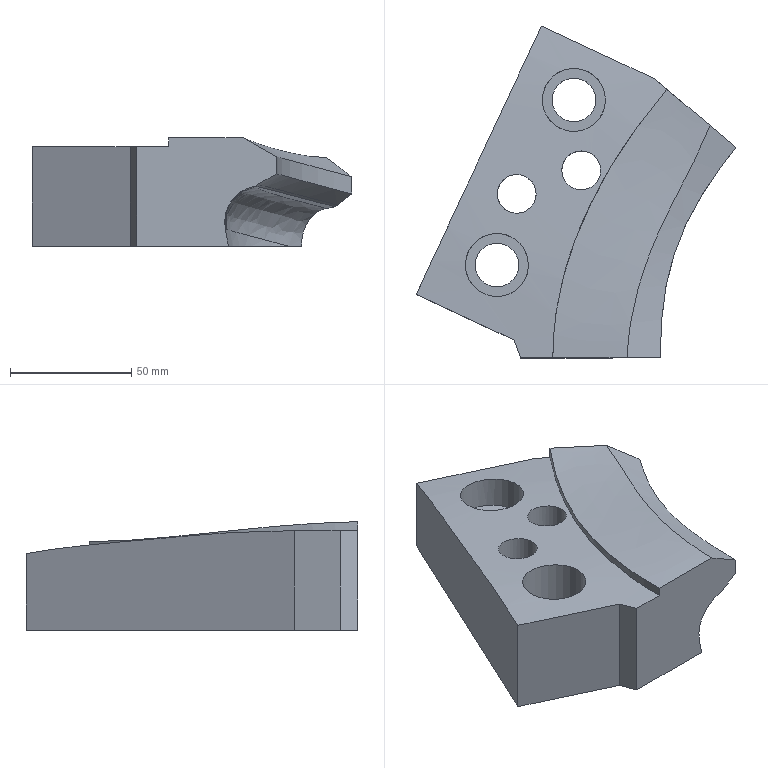Part | NX | features solid 2 | 1 solid | 25 faces | box 131.571 x 136.634 x 44.667 mm | volume 321257 mm3 | spline 10 | plane 9 | cylinder 6 | commonest cylinder face diameters 16 x2 18 x2 26 x2
STEP:
#1=CARTESIAN_POINT('',(-688.081,35.625,61.862));
#2=VERTEX_POINT('',#1);
#3=CARTESIAN_POINT('',(-693.271,39.979,61.591));
#4=VERTEX_POINT('',#3);
#5=CARTESIAN_POINT('',(-688.081,35.625,61.862));
#6=CARTESIAN_POINT('',(-689.811,37.076,61.773));
#7=CARTESIAN_POINT('',(-691.541,38.528,61.682));
#8=CARTESIAN_POINT('',(-693.271,39.979,61.591));
#9=B_SPLINE_CURVE_WITH_KNOTS('',3,(#5,#6,#7,#8),.UNSPECIFIED.,.F.,.F.,(4,4),(0.02865,0.03543),.UNSPECIFIED.);
#10=EDGE_CURVE('',#2,#4,#9,.T.);
#11=ORIENTED_EDGE('',*,*,#10,.F.);
#12=CARTESIAN_POINT('',(-688.081,35.625,66.502));
#13=VERTEX_POINT('',#12);
#14=CARTESIAN_POINT('',(-688.081,35.625,66.502));
#15=DIRECTION('',(0.,0.,1.));
#16=VECTOR('',#15,1000.);
#17=LINE('',#14,#16);
#18=EDGE_CURVE('',#2,#13,#17,.T.);
#19=ORIENTED_EDGE('',*,*,#18,.T.);
#20=CARTESIAN_POINT('',(-670.187,20.61,66.502));
#21=VERTEX_POINT('',#20);
#22=CARTESIAN_POINT('',(-688.081,35.625,66.502));
#23=CARTESIAN_POINT('',(-682.117,30.62,66.502));
#24=CARTESIAN_POINT('',(-676.152,25.615,66.502));
#25=CARTESIAN_POINT('',(-670.187,20.61,66.502));
#26=B_SPLINE_CURVE_WITH_KNOTS('',3,(#22,#23,#24,#25),.UNSPECIFIED.,.F.,.F.,(4,4),(0.006775,0.03013),.UNSPECIFIED.);
#27=EDGE_CURVE('',#13,#21,#26,.T.);
#28=ORIENTED_EDGE('',*,*,#27,.T.);
#29=CARTESIAN_POINT('',(-659.667,11.782,58.591));
#30=VERTEX_POINT('',#29);
#31=CARTESIAN_POINT('',(-670.187,20.61,66.502));
#32=CARTESIAN_POINT('',(-666.68,17.667,63.866));
#33=CARTESIAN_POINT('',(-663.173,14.724,61.229));
#34=CARTESIAN_POINT('',(-659.667,11.782,58.591));
#35=B_SPLINE_CURVE_WITH_KNOTS('',3,(#31,#32,#33,#34),.UNSPECIFIED.,.F.,.F.,(4,4),(0.001125,0.01697),.UNSPECIFIED.);
#36=EDGE_CURVE('',#21,#30,#35,.T.);
#37=ORIENTED_EDGE('',*,*,#36,.T.);
#38=CARTESIAN_POINT('',(-659.667,11.782,51.502));
#39=VERTEX_POINT('',#38);
#40=CARTESIAN_POINT('',(-659.667,11.782,58.342));
#41=DIRECTION('',(0.,0.,-1.));
#42=VECTOR('',#41,1000.);
#43=LINE('',#40,#42);
#44=EDGE_CURVE('',#30,#39,#43,.T.);
#45=ORIENTED_EDGE('',*,*,#44,.T.);
#46=CARTESIAN_POINT('',(-665.567,16.733,46.945));
#47=VERTEX_POINT('',#46);
#48=CARTESIAN_POINT('',(-665.567,16.733,46.945));
#49=CARTESIAN_POINT('',(-663.6,15.082,48.464));
#50=CARTESIAN_POINT('',(-661.633,13.432,49.982));
#51=CARTESIAN_POINT('',(-659.667,11.782,51.502));
#52=B_SPLINE_CURVE_WITH_KNOTS('',3,(#48,#49,#50,#51),.UNSPECIFIED.,.F.,.F.,(4,4),(0.,0.008949),.UNSPECIFIED.);
#53=EDGE_CURVE('',#47,#39,#52,.T.);
#54=ORIENTED_EDGE('',*,*,#53,.F.);
#55=CARTESIAN_POINT('',(-666.495,17.512,46.229));
#56=VERTEX_POINT('',#55);
#57=CARTESIAN_POINT('',(-666.495,17.512,46.229));
#58=CARTESIAN_POINT('',(-666.186,17.252,46.468));
#59=CARTESIAN_POINT('',(-665.876,16.992,46.706));
#60=CARTESIAN_POINT('',(-665.567,16.733,46.945));
#61=B_SPLINE_CURVE_WITH_KNOTS('',3,(#57,#58,#59,#60),.UNSPECIFIED.,.F.,.F.,(4,4),(0.03006,0.03147),.UNSPECIFIED.);
#62=EDGE_CURVE('',#56,#47,#61,.T.);
#63=ORIENTED_EDGE('',*,*,#62,.F.);
#64=CARTESIAN_POINT('',(-670.214,20.632,45.608));
#65=VERTEX_POINT('',#64);
#66=CARTESIAN_POINT('',(-670.214,20.632,45.608));
#67=CARTESIAN_POINT('',(-668.974,19.592,45.815));
#68=CARTESIAN_POINT('',(-667.734,18.552,46.022));
#69=CARTESIAN_POINT('',(-666.495,17.512,46.229));
#70=B_SPLINE_CURVE_WITH_KNOTS('',3,(#66,#67,#68,#69),.UNSPECIFIED.,.F.,.F.,(4,4),(0.001384,0.006278),.UNSPECIFIED.);
#71=EDGE_CURVE('',#65,#56,#70,.T.);
#72=ORIENTED_EDGE('',*,*,#71,.F.);
#73=CARTESIAN_POINT('',(-680.357,29.143,30.));
#74=VERTEX_POINT('',#73);
#75=CARTESIAN_POINT('',(-670.214,20.632,45.608));
#76=CARTESIAN_POINT('',(-673.081,23.038,45.129));
#77=CARTESIAN_POINT('',(-678.404,27.505,41.267));
#78=CARTESIAN_POINT('',(-680.437,29.211,33.749));
#79=CARTESIAN_POINT('',(-680.357,29.143,30.));
#80=B_SPLINE_CURVE_WITH_KNOTS('',3,(#75,#76,#77,#78,#79),.UNSPECIFIED.,.F.,.F.,(4,1,4),(0.,0.01116,0.02231),.UNSPECIFIED.);
#81=EDGE_CURVE('',#65,#74,#80,.T.);
#82=ORIENTED_EDGE('',*,*,#81,.T.);
#83=CARTESIAN_POINT('',(-693.271,39.979,30.));
#84=VERTEX_POINT('',#83);
#85=CARTESIAN_POINT('',(-734.044,74.192,30.));
#86=DIRECTION('',(-0.766,0.6428,0.));
#87=VECTOR('',#86,1000.);
#88=LINE('',#85,#87);
#89=EDGE_CURVE('',#74,#84,#88,.T.);
#90=ORIENTED_EDGE('',*,*,#89,.T.);
#91=CARTESIAN_POINT('',(-693.271,39.979,-162.739));
#92=DIRECTION('',(0.,0.,1.));
#93=VECTOR('',#92,1000.);
#94=LINE('',#91,#93);
#95=EDGE_CURVE('',#84,#4,#94,.T.);
#96=ORIENTED_EDGE('',*,*,#95,.T.);
#97=EDGE_LOOP('',(#11,#19,#28,#37,#45,#54,#63,#72,#82,#90,#96));
#98=FACE_BOUND('',#97,.T.);
#99=CARTESIAN_POINT('',(-734.044,74.192,-75.036));
#100=DIRECTION('',(-0.6428,-0.766,0.));
#101=DIRECTION('',(0.766,-0.6428,0.));
#102=AXIS2_PLACEMENT_3D('',#99,#100,#101);
#103=PLANE('',#102);
#104=ADVANCED_FACE('',(#98),#103,.F.);
#105=CARTESIAN_POINT('',(-735.,-75.,74.667));
#106=VERTEX_POINT('',#105);
#107=CARTESIAN_POINT('',(-704.43,-75.,74.667));
#108=VERTEX_POINT('',#107);
#109=CARTESIAN_POINT('',(-735.,-75.,74.667));
#110=CARTESIAN_POINT('',(-724.81,-75.,74.667));
#111=CARTESIAN_POINT('',(-714.62,-75.,74.667));
#112=CARTESIAN_POINT('',(-704.43,-75.,74.667));
#113=B_SPLINE_CURVE_WITH_KNOTS('',3,(#109,#110,#111,#112),.UNSPECIFIED.,.F.,.F.,(4,4),(0.01325,0.04382),.UNSPECIFIED.);
#114=EDGE_CURVE('',#106,#108,#113,.T.);
#115=ORIENTED_EDGE('',*,*,#114,.F.);
#116=CARTESIAN_POINT('',(-735.,-75.,70.988));
#117=VERTEX_POINT('',#116);
#118=CARTESIAN_POINT('',(-735.,-75.,74.667));
#119=DIRECTION('',(0.,0.,1.));
#120=VECTOR('',#119,1000.);
#121=LINE('',#118,#120);
#122=EDGE_CURVE('',#106,#117,#121,.F.);
#123=ORIENTED_EDGE('',*,*,#122,.T.);
#124=CARTESIAN_POINT('',(-748.254,-75.,71.092));
#125=VERTEX_POINT('',#124);
#126=CARTESIAN_POINT('',(-748.254,-75.,71.092));
#127=CARTESIAN_POINT('',(-743.836,-75.,71.066));
#128=CARTESIAN_POINT('',(-739.418,-75.,71.032));
#129=CARTESIAN_POINT('',(-735.,-75.,70.988));
#130=B_SPLINE_CURVE_WITH_KNOTS('',3,(#126,#127,#128,#129),.UNSPECIFIED.,.F.,.F.,(4,4),(0.,0.01325),.UNSPECIFIED.);
#131=EDGE_CURVE('',#125,#117,#130,.T.);
#132=ORIENTED_EDGE('',*,*,#131,.F.);
#133=CARTESIAN_POINT('',(-748.254,-75.,30.));
#134=VERTEX_POINT('',#133);
#135=CARTESIAN_POINT('',(-748.254,-75.,25.));
#136=DIRECTION('',(0.,0.,1.));
#137=VECTOR('',#136,1000.);
#138=LINE('',#135,#137);
#139=EDGE_CURVE('',#125,#134,#138,.F.);
#140=ORIENTED_EDGE('',*,*,#139,.T.);
#141=CARTESIAN_POINT('',(-710.465,-75.,30.));
#142=VERTEX_POINT('',#141);
#143=CARTESIAN_POINT('',(-775.,-75.,30.));
#144=DIRECTION('',(-1.,0.,0.));
#145=VECTOR('',#144,1000.);
#146=LINE('',#143,#145);
#147=EDGE_CURVE('',#142,#134,#146,.T.);
#148=ORIENTED_EDGE('',*,*,#147,.F.);
#149=CARTESIAN_POINT('',(-711.777,-75.,37.306));
#150=VERTEX_POINT('',#149);
#151=CARTESIAN_POINT('',(-710.465,-75.,30.));
#152=CARTESIAN_POINT('',(-710.902,-75.,32.435));
#153=CARTESIAN_POINT('',(-711.339,-75.,34.871));
#154=CARTESIAN_POINT('',(-711.777,-75.,37.306));
#155=B_SPLINE_CURVE_WITH_KNOTS('',3,(#151,#152,#153,#154),.UNSPECIFIED.,.F.,.F.,(4,4),(0.0254,0.03282),.UNSPECIFIED.);
#156=EDGE_CURVE('',#142,#150,#155,.T.);
#157=ORIENTED_EDGE('',*,*,#156,.T.);
#158=CARTESIAN_POINT('',(-699.604,-75.,54.73));
#159=VERTEX_POINT('',#158);
#160=CARTESIAN_POINT('',(-711.777,-75.,37.306));
#161=CARTESIAN_POINT('',(-712.127,-75.,39.26));
#162=CARTESIAN_POINT('',(-712.045,-75.,43.247));
#163=CARTESIAN_POINT('',(-709.633,-75.,48.776));
#164=CARTESIAN_POINT('',(-705.264,-75.,52.944));
#165=CARTESIAN_POINT('',(-701.56,-75.,54.387));
#166=CARTESIAN_POINT('',(-699.604,-75.,54.73));
#167=B_SPLINE_CURVE_WITH_KNOTS('',3,(#160,#161,#162,#163,#164,#165,#166),.UNSPECIFIED.,.F.,.F.,(4,1,1,1,4),(-0.01215,-0.006197,-0.0002407,0.005715,0.01167),.UNSPECIFIED.);
#168=EDGE_CURVE('',#159,#150,#167,.F.);
#169=ORIENTED_EDGE('',*,*,#168,.F.);
#170=CARTESIAN_POINT('',(-699.519,-75.,54.745));
#171=VERTEX_POINT('',#170);
#172=CARTESIAN_POINT('',(-699.604,-75.,54.73));
#173=CARTESIAN_POINT('',(-699.576,-75.,54.735));
#174=CARTESIAN_POINT('',(-699.547,-75.,54.74));
#175=CARTESIAN_POINT('',(-699.519,-75.,54.745));
#176=B_SPLINE_CURVE_WITH_KNOTS('',3,(#172,#173,#174,#175),.UNSPECIFIED.,.F.,.F.,(4,4),(0.004712,0.004798),.UNSPECIFIED.);
#177=EDGE_CURVE('',#159,#171,#176,.T.);
#178=ORIENTED_EDGE('',*,*,#177,.T.);
#179=CARTESIAN_POINT('',(-698.371,-75.,55.407));
#180=VERTEX_POINT('',#179);
#181=CARTESIAN_POINT('',(-699.518,-75.,54.745));
#182=CARTESIAN_POINT('',(-699.136,-75.,54.965));
#183=CARTESIAN_POINT('',(-698.753,-75.,55.186));
#184=CARTESIAN_POINT('',(-698.371,-75.,55.407));
#185=B_SPLINE_CURVE_WITH_KNOTS('',3,(#181,#182,#183,#184),.UNSPECIFIED.,.F.,.F.,(4,4),(0.04353,0.04486),.UNSPECIFIED.);
#186=EDGE_CURVE('',#171,#180,#185,.T.);
#187=ORIENTED_EDGE('',*,*,#186,.T.);
#188=CARTESIAN_POINT('',(-690.782,-75.,59.788));
#189=VERTEX_POINT('',#188);
#190=CARTESIAN_POINT('',(-698.371,-75.,55.407));
#191=CARTESIAN_POINT('',(-695.841,-75.,56.867));
#192=CARTESIAN_POINT('',(-693.311,-75.,58.328));
#193=CARTESIAN_POINT('',(-690.782,-75.,59.788));
#194=B_SPLINE_CURVE_WITH_KNOTS('',3,(#190,#191,#192,#193),.UNSPECIFIED.,.F.,.F.,(4,4),(0.,0.008763),.UNSPECIFIED.);
#195=EDGE_CURVE('',#180,#189,#194,.T.);
#196=ORIENTED_EDGE('',*,*,#195,.T.);
#197=CARTESIAN_POINT('',(-690.782,-75.,66.788));
#198=VERTEX_POINT('',#197);
#199=CARTESIAN_POINT('',(-690.782,-75.,59.186));
#200=DIRECTION('',(0.,0.,-1.));
#201=VECTOR('',#200,1000.);
#202=LINE('',#199,#201);
#203=EDGE_CURVE('',#198,#189,#202,.T.);
#204=ORIENTED_EDGE('',*,*,#203,.F.);
#205=CARTESIAN_POINT('',(-704.43,-75.,74.667));
#206=CARTESIAN_POINT('',(-699.88,-75.,72.041));
#207=CARTESIAN_POINT('',(-695.331,-75.,69.414));
#208=CARTESIAN_POINT('',(-690.782,-75.,66.788));
#209=B_SPLINE_CURVE_WITH_KNOTS('',3,(#205,#206,#207,#208),.UNSPECIFIED.,.F.,.F.,(4,4),(0.07485,0.09061),.UNSPECIFIED.);
#210=EDGE_CURVE('',#198,#108,#209,.F.);
#211=ORIENTED_EDGE('',*,*,#210,.T.);
#212=EDGE_LOOP('',(#115,#123,#132,#140,#148,#157,#169,#178,#187,#196,#204,#211));
#213=FACE_BOUND('',#212,.T.);
#214=CARTESIAN_POINT('',(-775.,-75.,69.026));
#215=DIRECTION('',(0.,-1.,0.));
#216=DIRECTION('',(1.,0.,0.));
#217=AXIS2_PLACEMENT_3D('',#214,#215,#216);
#218=PLANE('',#217);
#219=ADVANCED_FACE('',(#213),#218,.T.);
#220=CARTESIAN_POINT('',(-749.014,-36.777,30.));
#221=VERTEX_POINT('',#220);
#222=CARTESIAN_POINT('',(-758.014,-36.777,30.));
#223=DIRECTION('',(0.,0.,1.));
#224=DIRECTION('',(1.,0.,0.));
#225=AXIS2_PLACEMENT_3D('',#222,#223,#224);
#226=CIRCLE('',#225,9.);
#227=EDGE_CURVE('',#221,#221,#226,.T.);
#228=ORIENTED_EDGE('',*,*,#227,.T.);
#229=EDGE_LOOP('',(#228));
#230=FACE_BOUND('',#229,.T.);
#231=CARTESIAN_POINT('',(-741.867,-7.475,30.));
#232=VERTEX_POINT('',#231);
#233=CARTESIAN_POINT('',(-749.867,-7.475,30.));
#234=DIRECTION('',(0.,0.,1.));
#235=DIRECTION('',(1.,0.,0.));
#236=AXIS2_PLACEMENT_3D('',#233,#234,#235);
#237=CIRCLE('',#236,8.);
#238=EDGE_CURVE('',#232,#232,#237,.T.);
#239=ORIENTED_EDGE('',*,*,#238,.T.);
#240=EDGE_LOOP('',(#239));
#241=FACE_BOUND('',#240,.T.);
#242=CARTESIAN_POINT('',(-715.289,2.199,30.));
#243=VERTEX_POINT('',#242);
#244=CARTESIAN_POINT('',(-723.289,2.199,30.));
#245=DIRECTION('',(0.,0.,1.));
#246=DIRECTION('',(1.,0.,0.));
#247=AXIS2_PLACEMENT_3D('',#244,#245,#246);
#248=CIRCLE('',#247,8.);
#249=EDGE_CURVE('',#243,#243,#248,.T.);
#250=ORIENTED_EDGE('',*,*,#249,.T.);
#251=EDGE_LOOP('',(#250));
#252=FACE_BOUND('',#251,.T.);
#253=CARTESIAN_POINT('',(-717.318,31.196,30.));
#254=VERTEX_POINT('',#253);
#255=CARTESIAN_POINT('',(-726.318,31.196,30.));
#256=DIRECTION('',(0.,0.,1.));
#257=DIRECTION('',(1.,0.,0.));
#258=AXIS2_PLACEMENT_3D('',#255,#256,#257);
#259=CIRCLE('',#258,9.);
#260=EDGE_CURVE('',#254,#254,#259,.T.);
#261=ORIENTED_EDGE('',*,*,#260,.T.);
#262=EDGE_LOOP('',(#261));
#263=FACE_BOUND('',#262,.T.);
#264=CARTESIAN_POINT('',(-685.509,22.113,30.));
#265=VERTEX_POINT('',#264);
#266=CARTESIAN_POINT('',(-710.465,-75.,30.));
#267=CARTESIAN_POINT('',(-710.468,-70.804,30.));
#268=CARTESIAN_POINT('',(-710.485,-62.411,30.));
#269=CARTESIAN_POINT('',(-710.665,-45.619,30.));
#270=CARTESIAN_POINT('',(-709.623,-28.881,30.));
#271=CARTESIAN_POINT('',(-705.463,-14.264,30.));
#272=CARTESIAN_POINT('',(-702.162,-6.024,30.));
#273=CARTESIAN_POINT('',(-696.537,5.832,30.));
#274=CARTESIAN_POINT('',(-690.568,14.976,30.));
#275=CARTESIAN_POINT('',(-685.509,22.113,30.));
#276=B_SPLINE_CURVE_WITH_KNOTS('',3,(#266,#267,#268,#269,#270,#271,#272,#273,#274,#275),.UNSPECIFIED.,.F.,.F.,(4,1,1,1,1,1,1,4),(0.1678,0.1804,0.193,0.2182,0.2308,0.2371,0.2434,0.2685),.UNSPECIFIED.);
#277=EDGE_CURVE('',#142,#265,#276,.T.);
#278=ORIENTED_EDGE('',*,*,#277,.F.);
#279=ORIENTED_EDGE('',*,*,#147,.T.);
#280=CARTESIAN_POINT('',(-750.922,-67.668,30.));
#281=VERTEX_POINT('',#280);
#282=CARTESIAN_POINT('',(-750.797,-68.012,30.));
#283=DIRECTION('',(0.342,-0.9397,0.));
#284=VECTOR('',#283,1000.);
#285=LINE('',#282,#284);
#286=EDGE_CURVE('',#281,#134,#285,.T.);
#287=ORIENTED_EDGE('',*,*,#286,.F.);
#288=CARTESIAN_POINT('',(-791.237,-48.869,30.));
#289=VERTEX_POINT('',#288);
#290=CARTESIAN_POINT('',(-927.184,14.524,30.));
#291=DIRECTION('',(0.9063,-0.4226,0.));
#292=VECTOR('',#291,1000.);
#293=LINE('',#290,#292);
#294=EDGE_CURVE('',#281,#289,#293,.F.);
#295=ORIENTED_EDGE('',*,*,#294,.T.);
#296=CARTESIAN_POINT('',(-739.709,61.634,30.));
#297=VERTEX_POINT('',#296);
#298=CARTESIAN_POINT('',(-811.528,-92.383,30.));
#299=DIRECTION('',(0.4226,0.9063,0.));
#300=VECTOR('',#299,1000.);
#301=LINE('',#298,#300);
#302=EDGE_CURVE('',#289,#297,#301,.T.);
#303=ORIENTED_EDGE('',*,*,#302,.T.);
#304=CARTESIAN_POINT('',(-739.709,61.634,30.));
#305=DIRECTION('',(-0.9063,0.4226,0.));
#306=VECTOR('',#305,1000.);
#307=LINE('',#304,#306);
#308=EDGE_CURVE('',#84,#297,#307,.T.);
#309=ORIENTED_EDGE('',*,*,#308,.F.);
#310=ORIENTED_EDGE('',*,*,#89,.F.);
#311=CARTESIAN_POINT('',(-685.509,22.113,30.));
#312=CARTESIAN_POINT('',(-683.828,24.484,30.));
#313=CARTESIAN_POINT('',(-682.105,26.822,30.));
#314=CARTESIAN_POINT('',(-680.357,29.143,30.));
#315=B_SPLINE_CURVE_WITH_KNOTS('',3,(#311,#312,#313,#314),.UNSPECIFIED.,.F.,.F.,(4,4),(0.,0.008715),.UNSPECIFIED.);
#316=EDGE_CURVE('',#265,#74,#315,.T.);
#317=ORIENTED_EDGE('',*,*,#316,.F.);
#318=EDGE_LOOP('',(#278,#279,#287,#295,#303,#309,#310,#317));
#319=FACE_BOUND('',#318,.T.);
#320=CARTESIAN_POINT('',(-811.528,-92.383,30.));
#321=DIRECTION('',(0.,0.,1.));
#322=DIRECTION('',(1.,0.,0.));
#323=AXIS2_PLACEMENT_3D('',#320,#321,#322);
#324=PLANE('',#323);
#325=ADVANCED_FACE('',(#230,#241,#252,#263,#319),#324,.F.);
#326=ORIENTED_EDGE('',*,*,#186,.F.);
#327=CARTESIAN_POINT('',(-666.495,17.512,46.229));
#328=CARTESIAN_POINT('',(-671.574,10.867,47.54));
#329=CARTESIAN_POINT('',(-678.946,0.7357,49.507));
#330=CARTESIAN_POINT('',(-687.133,-13.802,51.643));
#331=CARTESIAN_POINT('',(-692.263,-25.496,52.98));
#332=CARTESIAN_POINT('',(-695.929,-37.581,53.926));
#333=CARTESIAN_POINT('',(-698.964,-53.96,54.682));
#334=CARTESIAN_POINT('',(-699.429,-66.563,54.759));
#335=CARTESIAN_POINT('',(-699.517,-75.,54.745));
#336=B_SPLINE_CURVE_WITH_KNOTS('',3,(#327,#328,#329,#330,#331,#332,#333,#334,#335),.UNSPECIFIED.,.F.,.F.,(4,1,1,1,1,1,4),(0.002498,0.02776,0.04039,0.05301,0.06564,0.07827,0.1035),.UNSPECIFIED.);
#337=EDGE_CURVE('',#171,#56,#336,.F.);
#338=ORIENTED_EDGE('',*,*,#337,.T.);
#339=ORIENTED_EDGE('',*,*,#62,.T.);
#340=CARTESIAN_POINT('',(-665.567,16.733,46.945));
#341=CARTESIAN_POINT('',(-670.344,10.46,48.191));
#342=CARTESIAN_POINT('',(-679.816,-2.401,50.683));
#343=CARTESIAN_POINT('',(-691.34,-24.269,53.703));
#344=CARTESIAN_POINT('',(-697.622,-48.974,55.319));
#345=CARTESIAN_POINT('',(-698.28,-66.27,55.42));
#346=CARTESIAN_POINT('',(-698.371,-75.,55.407));
#347=B_SPLINE_CURVE_WITH_KNOTS('',3,(#340,#341,#342,#343,#344,#345,#346),.UNSPECIFIED.,.F.,.F.,(4,1,1,1,4),(0.049,0.271,0.493,0.7149,0.9369),.UNSPECIFIED.);
#348=EDGE_CURVE('',#47,#180,#347,.T.);
#349=ORIENTED_EDGE('',*,*,#348,.T.);
#350=EDGE_LOOP('',(#326,#338,#339,#349));
#351=FACE_BOUND('',#350,.T.);
#352=CARTESIAN_POINT('',(-665.122,17.317,46.829));
#353=CARTESIAN_POINT('',(-666.181,17.984,46.118));
#354=CARTESIAN_POINT('',(-669.597,11.45,47.996));
#355=CARTESIAN_POINT('',(-670.662,12.108,47.285));
#356=CARTESIAN_POINT('',(-676.73,1.86,49.871));
#357=CARTESIAN_POINT('',(-677.821,2.475,49.16));
#358=CARTESIAN_POINT('',(-685.257,-12.625,52.109));
#359=CARTESIAN_POINT('',(-686.403,-12.123,51.395));
#360=CARTESIAN_POINT('',(-691.022,-25.333,53.616));
#361=CARTESIAN_POINT('',(-692.214,-24.953,52.899));
#362=CARTESIAN_POINT('',(-695.141,-38.936,54.682));
#363=CARTESIAN_POINT('',(-696.368,-38.696,53.963));
#364=CARTESIAN_POINT('',(-697.502,-53.144,55.266));
#365=CARTESIAN_POINT('',(-698.745,-53.031,54.547));
#366=CARTESIAN_POINT('',(-698.227,-65.447,55.41));
#367=CARTESIAN_POINT('',(-699.473,-65.406,54.69));
#368=CARTESIAN_POINT('',(-698.353,-72.992,55.411));
#369=CARTESIAN_POINT('',(-699.599,-72.974,54.691));
#370=CARTESIAN_POINT('',(-698.377,-75.643,55.406));
#371=CARTESIAN_POINT('',(-699.623,-75.63,54.686));
#372=B_SPLINE_SURFACE_WITH_KNOTS('',3,1,((#352,#353),(#354,#355),(#356,#357),(#358,#359),(#360,#361),(#362,#363),(#364,#365),(#366,#367),(#368,#369),(#370,#371)),.RULED_SURF.,.F.,.F.,.F.,(4,1,1,1,1,1,1,4),(2,2),(0.1893,0.2733,0.3239,0.3744,0.4249,0.4755,0.526,0.5532),(0.4382,0.4516),.UNSPECIFIED.);
#373=ADVANCED_FACE('',(#351),#372,.T.);
#374=ORIENTED_EDGE('',*,*,#18,.F.);
#375=CARTESIAN_POINT('',(-688.081,35.625,61.862));
#376=CARTESIAN_POINT('',(-691.354,31.724,62.615));
#377=CARTESIAN_POINT('',(-697.701,23.759,63.977));
#378=CARTESIAN_POINT('',(-706.568,11.197,65.417));
#379=CARTESIAN_POINT('',(-714.578,-1.929,66.652));
#380=CARTESIAN_POINT('',(-721.567,-15.632,67.897));
#381=CARTESIAN_POINT('',(-727.33,-29.882,69.173));
#382=CARTESIAN_POINT('',(-730.912,-42.029,70.064));
#383=CARTESIAN_POINT('',(-732.992,-51.975,70.549));
#384=CARTESIAN_POINT('',(-734.137,-59.551,70.63));
#385=CARTESIAN_POINT('',(-734.842,-67.257,70.764));
#386=CARTESIAN_POINT('',(-735.,-72.421,70.933));
#387=CARTESIAN_POINT('',(-735.,-75.,70.988));
#388=B_SPLINE_CURVE_WITH_KNOTS('',3,(#375,#376,#377,#378,#379,#380,#381,#382,#383,#384,#385,#386,#387),.UNSPECIFIED.,.F.,.F.,(4,1,1,1,1,1,1,1,1,1,4),(0.3255,0.341,0.3564,0.3719,0.3873,0.4027,0.4182,0.4259,0.4336,0.4413,0.4491),.UNSPECIFIED.);
#389=EDGE_CURVE('',#117,#2,#388,.F.);
#390=ORIENTED_EDGE('',*,*,#389,.F.);
#391=ORIENTED_EDGE('',*,*,#122,.F.);
#392=CARTESIAN_POINT('',(-688.081,35.625,66.502));
#393=CARTESIAN_POINT('',(-689.736,33.653,66.531));
#394=CARTESIAN_POINT('',(-692.993,29.668,66.546));
#395=CARTESIAN_POINT('',(-699.271,21.543,66.881));
#396=CARTESIAN_POINT('',(-709.615,6.863,67.871));
#397=CARTESIAN_POINT('',(-719.723,-11.034,69.771));
#398=CARTESIAN_POINT('',(-727.405,-30.091,71.777));
#399=CARTESIAN_POINT('',(-733.099,-49.528,73.586));
#400=CARTESIAN_POINT('',(-735.,-64.638,74.487));
#401=CARTESIAN_POINT('',(-735.,-75.,74.667));
#402=B_SPLINE_CURVE_WITH_KNOTS('',3,(#392,#393,#394,#395,#396,#397,#398,#399,#400,#401),.UNSPECIFIED.,.F.,.F.,(4,1,1,1,1,1,1,4),(0.001811,0.009513,0.01722,0.03262,0.06343,0.07883,0.09424,0.125),.UNSPECIFIED.);
#403=EDGE_CURVE('',#13,#106,#402,.T.);
#404=ORIENTED_EDGE('',*,*,#403,.F.);
#405=EDGE_LOOP('',(#374,#390,#391,#404));
#406=FACE_BOUND('',#405,.T.);
#407=CARTESIAN_POINT('',(-688.081,35.625,61.833));
#408=CARTESIAN_POINT('',(-688.081,35.625,66.672));
#409=CARTESIAN_POINT('',(-714.969,3.581,61.84));
#410=CARTESIAN_POINT('',(-714.969,3.581,66.679));
#411=CARTESIAN_POINT('',(-735.,-33.915,69.296));
#412=CARTESIAN_POINT('',(-735.,-33.915,74.134));
#413=CARTESIAN_POINT('',(-735.,-75.,69.999));
#414=CARTESIAN_POINT('',(-735.,-75.,74.838));
#415=B_SPLINE_SURFACE_WITH_KNOTS('',3,1,((#407,#408),(#409,#410),(#411,#412),(#413,#414)),.SURF_OF_LINEAR_EXTRUSION.,.F.,.F.,.F.,(4,4),(2,2),(0.000000002,1.),(0.,1.),.PIECEWISE_BEZIER_KNOTS.);
#416=ADVANCED_FACE('',(#406),#415,.T.);
#417=CARTESIAN_POINT('',(-739.709,61.634,61.591));
#418=VERTEX_POINT('',#417);
#419=CARTESIAN_POINT('',(-694.394,40.503,61.591));
#420=DIRECTION('',(0.9063,-0.4226,0.));
#421=VECTOR('',#420,1000.);
#422=LINE('',#419,#421);
#423=EDGE_CURVE('',#4,#418,#422,.F.);
#424=ORIENTED_EDGE('',*,*,#423,.F.);
#425=ORIENTED_EDGE('',*,*,#95,.F.);
#426=ORIENTED_EDGE('',*,*,#308,.T.);
#427=CARTESIAN_POINT('',(-739.709,61.634,65.));
#428=DIRECTION('',(0.,0.,-1.));
#429=VECTOR('',#428,1000.);
#430=LINE('',#427,#429);
#431=EDGE_CURVE('',#418,#297,#430,.T.);
#432=ORIENTED_EDGE('',*,*,#431,.F.);
#433=EDGE_LOOP('',(#424,#425,#426,#432));
#434=FACE_BOUND('',#433,.T.);
#435=CARTESIAN_POINT('',(-739.709,61.634,65.));
#436=DIRECTION('',(0.4226,0.9063,0.));
#437=DIRECTION('',(-0.9063,0.4226,0.));
#438=AXIS2_PLACEMENT_3D('',#435,#436,#437);
#439=PLANE('',#438);
#440=ADVANCED_FACE('',(#434),#439,.T.);
#441=CARTESIAN_POINT('',(-750.922,-67.668,70.99));
#442=VERTEX_POINT('',#441);
#443=CARTESIAN_POINT('',(-791.237,-48.869,70.99));
#444=VERTEX_POINT('',#443);
#445=CARTESIAN_POINT('',(-771.08,-58.269,70.99));
#446=DIRECTION('',(0.9063,-0.4226,0.));
#447=VECTOR('',#446,1000.);
#448=LINE('',#445,#447);
#449=EDGE_CURVE('',#442,#444,#448,.F.);
#450=ORIENTED_EDGE('',*,*,#449,.T.);
#451=CARTESIAN_POINT('',(-791.237,-48.869,65.));
#452=DIRECTION('',(0.,0.,1.));
#453=VECTOR('',#452,1000.);
#454=LINE('',#451,#453);
#455=EDGE_CURVE('',#444,#289,#454,.F.);
#456=ORIENTED_EDGE('',*,*,#455,.T.);
#457=ORIENTED_EDGE('',*,*,#294,.F.);
#458=CARTESIAN_POINT('',(-750.922,-67.668,65.989));
#459=DIRECTION('',(0.,0.,1.));
#460=VECTOR('',#459,1000.);
#461=LINE('',#458,#460);
#462=EDGE_CURVE('',#442,#281,#461,.F.);
#463=ORIENTED_EDGE('',*,*,#462,.F.);
#464=EDGE_LOOP('',(#450,#456,#457,#463));
#465=FACE_BOUND('',#464,.T.);
#466=CARTESIAN_POINT('',(-927.184,14.524,65.989));
#467=DIRECTION('',(0.4226,0.9063,0.));
#468=DIRECTION('',(0.9063,-0.4226,0.));
#469=AXIS2_PLACEMENT_3D('',#466,#467,#468);
#470=PLANE('',#469);
#471=ADVANCED_FACE('',(#465),#470,.F.);
#472=CARTESIAN_POINT('',(-739.709,61.634,61.591));
#473=CARTESIAN_POINT('',(-741.837,57.071,62.378));
#474=CARTESIAN_POINT('',(-746.1,47.927,63.815));
#475=CARTESIAN_POINT('',(-754.681,29.525,65.791));
#476=CARTESIAN_POINT('',(-763.274,11.098,67.338));
#477=CARTESIAN_POINT('',(-771.863,-7.321,69.044));
#478=CARTESIAN_POINT('',(-777.234,-18.839,69.973));
#479=CARTESIAN_POINT('',(-781.536,-28.066,70.507));
#480=CARTESIAN_POINT('',(-784.769,-34.999,70.635));
#481=CARTESIAN_POINT('',(-788.004,-41.935,70.741));
#482=CARTESIAN_POINT('',(-790.159,-46.557,70.931));
#483=CARTESIAN_POINT('',(-791.237,-48.869,70.99));
#484=B_SPLINE_CURVE_WITH_KNOTS('',3,(#472,#473,#474,#475,#476,#477,#478,#479,#480,#481,#482,#483),.UNSPECIFIED.,.F.,.F.,(4,1,1,1,1,1,1,1,1,4),(0.6336,0.6488,0.6641,0.6947,0.71,0.7253,0.7329,0.7406,0.7482,0.7558),.UNSPECIFIED.);
#485=EDGE_CURVE('',#444,#418,#484,.F.);
#486=ORIENTED_EDGE('',*,*,#485,.T.);
#487=ORIENTED_EDGE('',*,*,#431,.T.);
#488=ORIENTED_EDGE('',*,*,#302,.F.);
#489=ORIENTED_EDGE('',*,*,#455,.F.);
#490=EDGE_LOOP('',(#486,#487,#488,#489));
#491=FACE_BOUND('',#490,.T.);
#492=CARTESIAN_POINT('',(-811.528,-92.383,65.));
#493=DIRECTION('',(-0.9063,0.4226,0.));
#494=DIRECTION('',(-0.4226,-0.9063,0.));
#495=AXIS2_PLACEMENT_3D('',#492,#493,#494);
#496=PLANE('',#495);
#497=ADVANCED_FACE('',(#491),#496,.T.);
#498=CARTESIAN_POINT('',(-713.727,27.961,64.203));
#499=VERTEX_POINT('',#498);
#500=CARTESIAN_POINT('',(-718.973,18.799,65.249));
#501=CARTESIAN_POINT('',(-712.372,27.616,64.224));
#502=CARTESIAN_POINT('',(-713.901,38.499,63.075));
#503=CARTESIAN_POINT('',(-722.725,45.155,62.739));
#504=CARTESIAN_POINT('',(-733.651,43.591,63.579));
#505=CARTESIAN_POINT('',(-740.253,34.814,64.753));
#506=CARTESIAN_POINT('',(-738.749,23.908,65.565));
#507=CARTESIAN_POINT('',(-729.919,17.236,65.759));
#508=CARTESIAN_POINT('',(-718.973,18.799,65.249));
#509=CARTESIAN_POINT('',(-712.372,27.616,64.224));
#510=CARTESIAN_POINT('',(-713.901,38.499,63.075));
#511=B_SPLINE_CURVE_WITH_KNOTS('',3,(#500,#501,#502,#503,#504,#505,#506,#507,#508,#509,#510),.UNSPECIFIED.,.T.,.F.,(1,1,1,1,1,1,1,1,1,1,1,1,1,1,1),(-0.03056,-0.02038,-0.01019,0.,0.01019,0.02038,0.03056,0.04075,0.05094,0.06113,0.07131,0.0815,0.09169,0.1019,0.1121),.UNSPECIFIED.);
#512=EDGE_CURVE('',#499,#499,#511,.T.);
#513=ORIENTED_EDGE('',*,*,#512,.F.);
#514=EDGE_LOOP('',(#513));
#515=FACE_BOUND('',#514,.T.);
#516=CARTESIAN_POINT('',(-715.562,0.1264,66.536));
#517=VERTEX_POINT('',#516);
#518=CARTESIAN_POINT('',(-718.854,-5.478,67.057));
#519=CARTESIAN_POINT('',(-714.728,-0.09693,66.525));
#520=CARTESIAN_POINT('',(-715.607,6.624,66.059));
#521=CARTESIAN_POINT('',(-720.99,10.764,65.935));
#522=CARTESIAN_POINT('',(-727.726,9.874,66.238));
#523=CARTESIAN_POINT('',(-731.846,4.498,66.772));
#524=CARTESIAN_POINT('',(-730.977,-2.215,67.233));
#525=CARTESIAN_POINT('',(-725.591,-6.366,67.354));
#526=CARTESIAN_POINT('',(-718.854,-5.478,67.057));
#527=CARTESIAN_POINT('',(-714.728,-0.09693,66.525));
#528=CARTESIAN_POINT('',(-715.607,6.624,66.059));
#529=B_SPLINE_CURVE_WITH_KNOTS('',3,(#518,#519,#520,#521,#522,#523,#524,#525,#526,#527,#528),.UNSPECIFIED.,.T.,.F.,(1,1,1,1,1,1,1,1,1,1,1,1,1,1,1),(-0.01879,-0.01252,-0.006262,0.,0.006262,0.01252,0.01879,0.02505,0.03131,0.03757,0.04384,0.0501,0.05636,0.06262,0.06889),.UNSPECIFIED.);
#530=EDGE_CURVE('',#517,#517,#529,.T.);
#531=ORIENTED_EDGE('',*,*,#530,.F.);
#532=EDGE_LOOP('',(#531));
#533=FACE_BOUND('',#532,.T.);
#534=CARTESIAN_POINT('',(-742.142,-9.553,68.165));
#535=VERTEX_POINT('',#534);
#536=CARTESIAN_POINT('',(-745.438,-15.155,68.695));
#537=CARTESIAN_POINT('',(-741.308,-9.777,68.154));
#538=CARTESIAN_POINT('',(-742.182,-3.056,67.681));
#539=CARTESIAN_POINT('',(-747.562,1.089,67.56));
#540=CARTESIAN_POINT('',(-754.299,0.2037,67.86));
#541=CARTESIAN_POINT('',(-758.423,-5.169,68.406));
#542=CARTESIAN_POINT('',(-757.559,-11.883,68.867));
#543=CARTESIAN_POINT('',(-752.176,-16.038,68.983));
#544=CARTESIAN_POINT('',(-745.438,-15.155,68.695));
#545=CARTESIAN_POINT('',(-741.308,-9.777,68.154));
#546=CARTESIAN_POINT('',(-742.182,-3.056,67.681));
#547=B_SPLINE_CURVE_WITH_KNOTS('',3,(#536,#537,#538,#539,#540,#541,#542,#543,#544,#545,#546),.UNSPECIFIED.,.T.,.F.,(1,1,1,1,1,1,1,1,1,1,1,1,1,1,1),(-0.01879,-0.01253,-0.006263,0.,0.006263,0.01253,0.01879,0.02505,0.03131,0.03758,0.04384,0.0501,0.05636,0.06263,0.06889),.UNSPECIFIED.);
#548=EDGE_CURVE('',#535,#535,#547,.T.);
#549=ORIENTED_EDGE('',*,*,#548,.F.);
#550=EDGE_LOOP('',(#549));
#551=FACE_BOUND('',#550,.T.);
#552=CARTESIAN_POINT('',(-745.338,-39.66,70.246));
#553=VERTEX_POINT('',#552);
#554=CARTESIAN_POINT('',(-750.347,-48.978,70.659));
#555=CARTESIAN_POINT('',(-743.965,-39.967,70.287));
#556=CARTESIAN_POINT('',(-745.821,-29.11,69.671));
#557=CARTESIAN_POINT('',(-754.807,-22.732,69.526));
#558=CARTESIAN_POINT('',(-765.677,-24.578,69.977));
#559=CARTESIAN_POINT('',(-772.056,-33.564,70.572));
#560=CARTESIAN_POINT('',(-770.22,-44.429,70.654));
#561=CARTESIAN_POINT('',(-761.228,-50.822,70.668));
#562=CARTESIAN_POINT('',(-750.347,-48.978,70.659));
#563=CARTESIAN_POINT('',(-743.965,-39.967,70.287));
#564=CARTESIAN_POINT('',(-745.821,-29.11,69.671));
#565=B_SPLINE_CURVE_WITH_KNOTS('',3,(#554,#555,#556,#557,#558,#559,#560,#561,#562,#563,#564),.UNSPECIFIED.,.T.,.F.,(1,1,1,1,1,1,1,1,1,1,1,1,1,1,1),(-0.03049,-0.02033,-0.01016,0.,0.01016,0.02033,0.03049,0.04066,0.05082,0.06099,0.07115,0.08132,0.09148,0.1016,0.1118),.UNSPECIFIED.);
#566=EDGE_CURVE('',#553,#553,#565,.T.);
#567=ORIENTED_EDGE('',*,*,#566,.F.);
#568=EDGE_LOOP('',(#567));
#569=FACE_BOUND('',#568,.T.);
#570=ORIENTED_EDGE('',*,*,#389,.T.);
#571=ORIENTED_EDGE('',*,*,#10,.T.);
#572=ORIENTED_EDGE('',*,*,#423,.T.);
#573=ORIENTED_EDGE('',*,*,#485,.F.);
#574=ORIENTED_EDGE('',*,*,#449,.F.);
#575=CARTESIAN_POINT('',(-748.254,-75.,71.092));
#576=CARTESIAN_POINT('',(-749.143,-72.556,71.066));
#577=CARTESIAN_POINT('',(-750.033,-70.112,71.033));
#578=CARTESIAN_POINT('',(-750.922,-67.668,70.99));
#579=B_SPLINE_CURVE_WITH_KNOTS('',3,(#575,#576,#577,#578),.UNSPECIFIED.,.F.,.F.,(4,4),(0.01488,0.02268),.UNSPECIFIED.);
#580=EDGE_CURVE('',#125,#442,#579,.T.);
#581=ORIENTED_EDGE('',*,*,#580,.F.);
#582=ORIENTED_EDGE('',*,*,#131,.T.);
#583=EDGE_LOOP('',(#570,#571,#572,#573,#574,#581,#582));
#584=FACE_BOUND('',#583,.T.);
#585=CARTESIAN_POINT('',(-791.241,-55.742,71.101));
#586=CARTESIAN_POINT('',(-723.212,-87.464,71.101));
#587=CARTESIAN_POINT('',(-791.361,-52.934,71.07));
#588=CARTESIAN_POINT('',(-723.331,-84.657,71.07));
#589=CARTESIAN_POINT('',(-791.679,-47.319,70.98));
#590=CARTESIAN_POINT('',(-723.65,-79.042,70.98));
#591=CARTESIAN_POINT('',(-792.389,-40.333,70.773));
#592=CARTESIAN_POINT('',(-724.359,-72.056,70.773));
#593=CARTESIAN_POINT('',(-792.765,-34.805,70.656));
#594=CARTESIAN_POINT('',(-724.736,-66.527,70.656));
#595=CARTESIAN_POINT('',(-792.793,-30.626,70.631));
#596=CARTESIAN_POINT('',(-724.763,-62.348,70.631));
#597=CARTESIAN_POINT('',(-792.711,-26.377,70.574));
#598=CARTESIAN_POINT('',(-724.681,-58.099,70.574));
#599=CARTESIAN_POINT('',(-792.598,-20.725,70.4));
#600=CARTESIAN_POINT('',(-724.568,-52.447,70.4));
#601=CARTESIAN_POINT('',(-792.306,-13.696,70.061));
#602=CARTESIAN_POINT('',(-724.277,-45.418,70.061));
#603=CARTESIAN_POINT('',(-791.289,-2.519,69.34));
#604=CARTESIAN_POINT('',(-723.26,-34.241,69.34));
#605=CARTESIAN_POINT('',(-788.668,11.247,68.234));
#606=CARTESIAN_POINT('',(-720.638,-20.475,68.234));
#607=CARTESIAN_POINT('',(-782.849,26.991,66.859));
#608=CARTESIAN_POINT('',(-714.82,-4.732,66.859));
#609=CARTESIAN_POINT('',(-774.594,41.613,65.523));
#610=CARTESIAN_POINT('',(-706.565,9.89,65.523));
#611=CARTESIAN_POINT('',(-764.862,55.338,63.973));
#612=CARTESIAN_POINT('',(-696.833,23.616,63.973));
#613=CARTESIAN_POINT('',(-758.043,64.211,62.437));
#614=CARTESIAN_POINT('',(-690.014,32.488,62.437));
#615=CARTESIAN_POINT('',(-754.592,68.574,61.591));
#616=CARTESIAN_POINT('',(-686.563,36.851,61.591));
#617=B_SPLINE_SURFACE_WITH_KNOTS('',3,1,((#585,#586),(#587,#588),(#589,#590),(#591,#592),(#593,#594),(#595,#596),(#597,#598),(#599,#600),(#601,#602),(#603,#604),(#605,#606),(#607,#608),(#609,#610),(#611,#612),(#613,#614),(#615,#616)),.SURF_OF_LINEAR_EXTRUSION.,.F.,.F.,.F.,(4,1,1,1,1,1,1,1,1,1,1,1,1,4),(2,2),(0.1522,0.205,0.2578,0.2842,0.3106,0.337,0.3634,0.4162,0.469,0.5746,0.6802,0.7858,0.8914,0.997),(0.,1.),.UNSPECIFIED.);
#618=ADVANCED_FACE('',(#515,#533,#551,#569,#584),#617,.F.);
#619=ORIENTED_EDGE('',*,*,#580,.T.);
#620=ORIENTED_EDGE('',*,*,#462,.T.);
#621=ORIENTED_EDGE('',*,*,#286,.T.);
#622=ORIENTED_EDGE('',*,*,#139,.F.);
#623=EDGE_LOOP('',(#619,#620,#621,#622));
#624=FACE_BOUND('',#623,.T.);
#625=CARTESIAN_POINT('',(-750.797,-68.012,65.989));
#626=DIRECTION('',(0.9397,0.342,0.));
#627=DIRECTION('',(0.342,-0.9397,0.));
#628=AXIS2_PLACEMENT_3D('',#625,#626,#627);
#629=PLANE('',#628);
#630=ADVANCED_FACE('',(#624),#629,.F.);
#631=CARTESIAN_POINT('',(-767.014,-36.777,50.));
#632=VERTEX_POINT('',#631);
#633=CARTESIAN_POINT('',(-758.014,-36.777,50.));
#634=DIRECTION('',(0.,0.,-1.));
#635=DIRECTION('',(-1.,0.,0.));
#636=AXIS2_PLACEMENT_3D('',#633,#634,#635);
#637=CIRCLE('',#636,9.);
#638=EDGE_CURVE('',#632,#632,#637,.T.);
#639=ORIENTED_EDGE('',*,*,#638,.F.);
#640=EDGE_LOOP('',(#639));
#641=FACE_BOUND('',#640,.T.);
#642=ORIENTED_EDGE('',*,*,#227,.F.);
#643=EDGE_LOOP('',(#642));
#644=FACE_BOUND('',#643,.T.);
#645=CARTESIAN_POINT('',(-758.014,-36.777,40.));
#646=DIRECTION('',(0.,0.,-1.));
#647=DIRECTION('',(-1.,0.,0.));
#648=AXIS2_PLACEMENT_3D('',#645,#646,#647);
#649=CYLINDRICAL_SURFACE('',#648,9.);
#650=ADVANCED_FACE('',(#641,#644),#649,.F.);
#651=ORIENTED_EDGE('',*,*,#638,.T.);
#652=EDGE_LOOP('',(#651));
#653=FACE_BOUND('',#652,.T.);
#654=CARTESIAN_POINT('',(-771.014,-36.777,50.));
#655=VERTEX_POINT('',#654);
#656=CARTESIAN_POINT('',(-758.014,-36.777,50.));
#657=DIRECTION('',(0.,0.,-1.));
#658=DIRECTION('',(-1.,0.,0.));
#659=AXIS2_PLACEMENT_3D('',#656,#657,#658);
#660=CIRCLE('',#659,13.);
#661=EDGE_CURVE('',#655,#655,#660,.F.);
#662=ORIENTED_EDGE('',*,*,#661,.T.);
#663=EDGE_LOOP('',(#662));
#664=FACE_BOUND('',#663,.T.);
#665=CARTESIAN_POINT('',(-758.014,-36.777,50.));
#666=DIRECTION('',(0.,0.,-1.));
#667=DIRECTION('',(-1.,0.,0.));
#668=AXIS2_PLACEMENT_3D('',#665,#666,#667);
#669=PLANE('',#668);
#670=ADVANCED_FACE('',(#653,#664),#669,.F.);
#671=ORIENTED_EDGE('',*,*,#566,.T.);
#672=EDGE_LOOP('',(#671));
#673=FACE_BOUND('',#672,.T.);
#674=ORIENTED_EDGE('',*,*,#661,.F.);
#675=EDGE_LOOP('',(#674));
#676=FACE_BOUND('',#675,.T.);
#677=CARTESIAN_POINT('',(-758.014,-36.777,40.));
#678=DIRECTION('',(0.,0.,1.));
#679=DIRECTION('',(1.,0.,0.));
#680=AXIS2_PLACEMENT_3D('',#677,#678,#679);
#681=CYLINDRICAL_SURFACE('',#680,13.);
#682=ADVANCED_FACE('',(#673,#676),#681,.F.);
#683=ORIENTED_EDGE('',*,*,#548,.T.);
#684=EDGE_LOOP('',(#683));
#685=FACE_BOUND('',#684,.T.);
#686=ORIENTED_EDGE('',*,*,#238,.F.);
#687=EDGE_LOOP('',(#686));
#688=FACE_BOUND('',#687,.T.);
#689=CARTESIAN_POINT('',(-749.867,-7.475,25.));
#690=DIRECTION('',(0.,0.,1.));
#691=DIRECTION('',(1.,0.,0.));
#692=AXIS2_PLACEMENT_3D('',#689,#690,#691);
#693=CYLINDRICAL_SURFACE('',#692,8.);
#694=ADVANCED_FACE('',(#685,#688),#693,.F.);
#695=ORIENTED_EDGE('',*,*,#530,.T.);
#696=EDGE_LOOP('',(#695));
#697=FACE_BOUND('',#696,.T.);
#698=ORIENTED_EDGE('',*,*,#249,.F.);
#699=EDGE_LOOP('',(#698));
#700=FACE_BOUND('',#699,.T.);
#701=CARTESIAN_POINT('',(-723.289,2.199,25.));
#702=DIRECTION('',(0.,0.,1.));
#703=DIRECTION('',(1.,0.,0.));
#704=AXIS2_PLACEMENT_3D('',#701,#702,#703);
#705=CYLINDRICAL_SURFACE('',#704,8.);
#706=ADVANCED_FACE('',(#697,#700),#705,.F.);
#707=CARTESIAN_POINT('',(-735.318,31.196,50.));
#708=VERTEX_POINT('',#707);
#709=CARTESIAN_POINT('',(-726.318,31.196,50.));
#710=DIRECTION('',(0.,0.,-1.));
#711=DIRECTION('',(-1.,0.,0.));
#712=AXIS2_PLACEMENT_3D('',#709,#710,#711);
#713=CIRCLE('',#712,9.);
#714=EDGE_CURVE('',#708,#708,#713,.T.);
#715=ORIENTED_EDGE('',*,*,#714,.F.);
#716=EDGE_LOOP('',(#715));
#717=FACE_BOUND('',#716,.T.);
#718=ORIENTED_EDGE('',*,*,#260,.F.);
#719=EDGE_LOOP('',(#718));
#720=FACE_BOUND('',#719,.T.);
#721=CARTESIAN_POINT('',(-726.318,31.196,40.));
#722=DIRECTION('',(0.,0.,-1.));
#723=DIRECTION('',(-1.,0.,0.));
#724=AXIS2_PLACEMENT_3D('',#721,#722,#723);
#725=CYLINDRICAL_SURFACE('',#724,9.);
#726=ADVANCED_FACE('',(#717,#720),#725,.F.);
#727=ORIENTED_EDGE('',*,*,#714,.T.);
#728=EDGE_LOOP('',(#727));
#729=FACE_BOUND('',#728,.T.);
#730=CARTESIAN_POINT('',(-739.318,31.196,50.));
#731=VERTEX_POINT('',#730);
#732=CARTESIAN_POINT('',(-726.318,31.196,50.));
#733=DIRECTION('',(0.,0.,-1.));
#734=DIRECTION('',(-1.,0.,0.));
#735=AXIS2_PLACEMENT_3D('',#732,#733,#734);
#736=CIRCLE('',#735,13.);
#737=EDGE_CURVE('',#731,#731,#736,.F.);
#738=ORIENTED_EDGE('',*,*,#737,.T.);
#739=EDGE_LOOP('',(#738));
#740=FACE_BOUND('',#739,.T.);
#741=CARTESIAN_POINT('',(-726.318,31.196,50.));
#742=DIRECTION('',(0.,0.,-1.));
#743=DIRECTION('',(-1.,0.,0.));
#744=AXIS2_PLACEMENT_3D('',#741,#742,#743);
#745=PLANE('',#744);
#746=ADVANCED_FACE('',(#729,#740),#745,.F.);
#747=ORIENTED_EDGE('',*,*,#512,.T.);
#748=EDGE_LOOP('',(#747));
#749=FACE_BOUND('',#748,.T.);
#750=ORIENTED_EDGE('',*,*,#737,.F.);
#751=EDGE_LOOP('',(#750));
#752=FACE_BOUND('',#751,.T.);
#753=CARTESIAN_POINT('',(-726.318,31.196,40.));
#754=DIRECTION('',(0.,0.,1.));
#755=DIRECTION('',(1.,0.,0.));
#756=AXIS2_PLACEMENT_3D('',#753,#754,#755);
#757=CYLINDRICAL_SURFACE('',#756,13.);
#758=ADVANCED_FACE('',(#749,#752),#757,.F.);
#759=CARTESIAN_POINT('',(-690.782,-75.,66.788));
#760=CARTESIAN_POINT('',(-690.726,-71.039,66.801));
#761=CARTESIAN_POINT('',(-690.591,-63.122,66.763));
#762=CARTESIAN_POINT('',(-689.535,-51.349,66.575));
#763=CARTESIAN_POINT('',(-687.412,-39.739,66.034));
#764=CARTESIAN_POINT('',(-683.883,-28.239,65.082));
#765=CARTESIAN_POINT('',(-679.103,-17.486,63.78));
#766=CARTESIAN_POINT('',(-671.36,-3.948,61.725));
#767=CARTESIAN_POINT('',(-664.407,5.541,59.85));
#768=CARTESIAN_POINT('',(-659.667,11.782,58.591));
#769=B_SPLINE_CURVE_WITH_KNOTS('',3,(#759,#760,#761,#762,#763,#764,#765,#766,#767,#768),.UNSPECIFIED.,.F.,.F.,(4,1,1,1,1,1,1,4),(0.002814,0.01462,0.02643,0.03824,0.05005,0.06186,0.07367,0.09729),.UNSPECIFIED.);
#770=EDGE_CURVE('',#198,#30,#769,.T.);
#771=ORIENTED_EDGE('',*,*,#770,.F.);
#772=ORIENTED_EDGE('',*,*,#203,.T.);
#773=CARTESIAN_POINT('',(-690.782,-75.,59.788));
#774=CARTESIAN_POINT('',(-690.725,-71.022,59.803));
#775=CARTESIAN_POINT('',(-690.589,-63.071,59.764));
#776=CARTESIAN_POINT('',(-689.525,-51.246,59.572));
#777=CARTESIAN_POINT('',(-687.365,-39.534,59.006));
#778=CARTESIAN_POINT('',(-682.627,-24.226,57.702));
#779=CARTESIAN_POINT('',(-673.64,-7.059,55.257));
#780=CARTESIAN_POINT('',(-664.396,5.556,52.754));
#781=CARTESIAN_POINT('',(-659.667,11.782,51.502));
#782=B_SPLINE_CURVE_WITH_KNOTS('',3,(#773,#774,#775,#776,#777,#778,#779,#780,#781),.UNSPECIFIED.,.F.,.F.,(4,1,1,1,1,1,4),(0.002818,0.01469,0.02657,0.03844,0.05032,0.07407,0.09782),.UNSPECIFIED.);
#783=EDGE_CURVE('',#189,#39,#782,.T.);
#784=ORIENTED_EDGE('',*,*,#783,.T.);
#785=ORIENTED_EDGE('',*,*,#44,.F.);
#786=EDGE_LOOP('',(#771,#772,#784,#785));
#787=FACE_BOUND('',#786,.T.);
#788=CARTESIAN_POINT('',(-659.667,11.782,66.924));
#789=CARTESIAN_POINT('',(-659.667,11.782,51.41));
#790=CARTESIAN_POINT('',(-664.425,5.518,66.924));
#791=CARTESIAN_POINT('',(-664.425,5.518,51.41));
#792=CARTESIAN_POINT('',(-673.745,-7.176,66.924));
#793=CARTESIAN_POINT('',(-673.745,-7.176,51.41));
#794=CARTESIAN_POINT('',(-684.673,-28.25,66.924));
#795=CARTESIAN_POINT('',(-684.673,-28.25,51.41));
#796=CARTESIAN_POINT('',(-689.211,-47.516,66.924));
#797=CARTESIAN_POINT('',(-689.211,-47.516,51.41));
#798=CARTESIAN_POINT('',(-690.591,-63.199,66.924));
#799=CARTESIAN_POINT('',(-690.591,-63.199,51.41));
#800=CARTESIAN_POINT('',(-690.726,-71.066,66.924));
#801=CARTESIAN_POINT('',(-690.726,-71.066,51.41));
#802=CARTESIAN_POINT('',(-690.782,-75.,66.924));
#803=CARTESIAN_POINT('',(-690.782,-75.,51.41));
#804=B_SPLINE_SURFACE_WITH_KNOTS('',3,1,((#788,#789),(#790,#791),(#792,#793),(#794,#795),(#796,#797),(#798,#799),(#800,#801),(#802,#803)),.SURF_OF_LINEAR_EXTRUSION.,.F.,.F.,.F.,(4,1,1,1,1,4),(2,2),(0.1516,0.1571,0.1626,0.1681,0.1708,0.1736),(0.,1.),.UNSPECIFIED.);
#805=ADVANCED_FACE('',(#787),#804,.T.);
#806=ORIENTED_EDGE('',*,*,#195,.F.);
#807=ORIENTED_EDGE('',*,*,#348,.F.);
#808=ORIENTED_EDGE('',*,*,#53,.T.);
#809=ORIENTED_EDGE('',*,*,#783,.F.);
#810=EDGE_LOOP('',(#806,#807,#808,#809));
#811=FACE_BOUND('',#810,.T.);
#812=CARTESIAN_POINT('',(-658.627,13.036,51.281));
#813=CARTESIAN_POINT('',(-665.223,17.184,46.855));
#814=CARTESIAN_POINT('',(-663.034,7.265,52.44));
#815=CARTESIAN_POINT('',(-669.665,11.36,48.014));
#816=CARTESIAN_POINT('',(-669.966,-2.021,54.312));
#817=CARTESIAN_POINT('',(-676.759,1.81,49.879));
#818=CARTESIAN_POINT('',(-678.121,-15.751,56.557));
#819=CARTESIAN_POINT('',(-685.257,-12.625,52.109));
#820=CARTESIAN_POINT('',(-683.602,-27.694,58.078));
#821=CARTESIAN_POINT('',(-691.022,-25.333,53.616));
#822=CARTESIAN_POINT('',(-687.506,-40.428,59.156));
#823=CARTESIAN_POINT('',(-695.141,-38.936,54.682));
#824=CARTESIAN_POINT('',(-689.763,-53.849,59.746));
#825=CARTESIAN_POINT('',(-697.502,-53.144,55.266));
#826=CARTESIAN_POINT('',(-690.469,-65.692,59.89));
#827=CARTESIAN_POINT('',(-698.227,-65.442,55.41));
#828=CARTESIAN_POINT('',(-690.593,-73.094,59.891));
#829=CARTESIAN_POINT('',(-698.353,-72.983,55.411));
#830=CARTESIAN_POINT('',(-690.617,-75.707,59.886));
#831=CARTESIAN_POINT('',(-698.377,-75.629,55.406));
#832=B_SPLINE_SURFACE_WITH_KNOTS('',3,1,((#812,#813),(#814,#815),(#816,#817),(#818,#819),(#820,#821),(#822,#823),(#824,#825),(#826,#827),(#828,#829),(#830,#831)),.RULED_SURF.,.F.,.F.,.F.,(4,1,1,1,1,1,1,4),(2,2),(0.04367,0.25,0.375,0.5,0.625,0.75,0.875,0.9422),(-0.3528,0.),.UNSPECIFIED.);
#833=ADVANCED_FACE('',(#811),#832,.T.);
#834=ORIENTED_EDGE('',*,*,#277,.T.);
#835=CARTESIAN_POINT('',(-711.777,-75.,37.306));
#836=CARTESIAN_POINT('',(-711.777,-70.661,37.313));
#837=CARTESIAN_POINT('',(-711.787,-61.984,37.264));
#838=CARTESIAN_POINT('',(-711.75,-48.964,37.105));
#839=CARTESIAN_POINT('',(-710.956,-35.979,36.791));
#840=CARTESIAN_POINT('',(-708.813,-23.339,36.181));
#841=CARTESIAN_POINT('',(-704.999,-11.077,35.152));
#842=CARTESIAN_POINT('',(-697.7,4.721,33.217));
#843=CARTESIAN_POINT('',(-690.556,15.258,31.324));
#844=CARTESIAN_POINT('',(-685.509,22.113,30.));
#845=B_SPLINE_CURVE_WITH_KNOTS('',3,(#835,#836,#837,#838,#839,#840,#841,#842,#843,#844),.UNSPECIFIED.,.F.,.F.,(4,1,1,1,1,1,1,4),(-0.005713,0.007303,0.02032,0.03333,0.04635,0.05937,0.07238,0.09841),.UNSPECIFIED.);
#846=EDGE_CURVE('',#150,#265,#845,.T.);
#847=ORIENTED_EDGE('',*,*,#846,.F.);
#848=ORIENTED_EDGE('',*,*,#156,.F.);
#849=EDGE_LOOP('',(#834,#847,#848));
#850=FACE_BOUND('',#849,.T.);
#851=CARTESIAN_POINT('',(-685.136,22.628,29.946));
#852=CARTESIAN_POINT('',(-687.775,19.056,30.639));
#853=CARTESIAN_POINT('',(-690.33,15.466,31.314));
#854=CARTESIAN_POINT('',(-696.607,5.871,32.979));
#855=CARTESIAN_POINT('',(-700.075,-0.2942,33.903));
#856=CARTESIAN_POINT('',(-705.732,-13.131,35.443));
#857=CARTESIAN_POINT('',(-707.87,-19.797,36.05));
#858=CARTESIAN_POINT('',(-710.679,-33.49,36.91));
#859=CARTESIAN_POINT('',(-711.345,-40.485,37.163));
#860=CARTESIAN_POINT('',(-711.881,-54.694,37.414));
#861=CARTESIAN_POINT('',(-711.793,-61.933,37.416));
#862=CARTESIAN_POINT('',(-711.79,-69.287,37.39));
#863=CARTESIAN_POINT('',(-711.789,-71.416,37.382));
#864=CARTESIAN_POINT('',(-711.789,-73.545,37.375));
#865=CARTESIAN_POINT('',(-711.788,-75.674,37.367));
#866=CARTESIAN_POINT('',(-685.122,21.658,24.996));
#867=CARTESIAN_POINT('',(-687.751,18.097,25.686));
#868=CARTESIAN_POINT('',(-690.287,14.529,26.357));
#869=CARTESIAN_POINT('',(-696.491,5.014,28.009));
#870=CARTESIAN_POINT('',(-699.898,-1.084,28.923));
#871=CARTESIAN_POINT('',(-705.408,-13.758,30.447));
#872=CARTESIAN_POINT('',(-707.455,-20.322,31.048));
#873=CARTESIAN_POINT('',(-710.076,-33.802,31.909));
#874=CARTESIAN_POINT('',(-710.645,-40.685,32.171));
#875=CARTESIAN_POINT('',(-711.038,-54.729,32.44));
#876=CARTESIAN_POINT('',(-710.91,-61.92,32.45));
#877=CARTESIAN_POINT('',(-710.902,-69.269,32.424));
#878=CARTESIAN_POINT('',(-710.9,-71.397,32.417));
#879=CARTESIAN_POINT('',(-710.898,-73.524,32.41));
#880=CARTESIAN_POINT('',(-710.896,-75.652,32.402));
#881=CARTESIAN_POINT('',(-685.115,21.166,22.482));
#882=CARTESIAN_POINT('',(-687.739,17.611,23.171));
#883=CARTESIAN_POINT('',(-690.265,14.053,23.84));
#884=CARTESIAN_POINT('',(-696.433,4.578,25.485));
#885=CARTESIAN_POINT('',(-699.808,-1.486,26.394));
#886=CARTESIAN_POINT('',(-705.244,-14.077,27.91));
#887=CARTESIAN_POINT('',(-707.244,-20.588,28.508));
#888=CARTESIAN_POINT('',(-709.77,-33.96,29.37));
#889=CARTESIAN_POINT('',(-710.289,-40.786,29.635));
#890=CARTESIAN_POINT('',(-710.61,-54.747,29.913));
#891=CARTESIAN_POINT('',(-710.461,-61.913,29.927));
#892=CARTESIAN_POINT('',(-710.452,-69.26,29.902));
#893=CARTESIAN_POINT('',(-710.449,-71.387,29.895));
#894=CARTESIAN_POINT('',(-710.446,-73.514,29.888));
#895=CARTESIAN_POINT('',(-710.444,-75.641,29.881));
#896=B_SPLINE_SURFACE_WITH_KNOTS('',1,3,((#851,#852,#853,#854,#855,#856,#857,#858,#859,#860,#861,#862,#863,#864,#865),(#866,#867,#868,#869,#870,#871,#872,#873,#874,#875,#876,#877,#878,#879,#880),(#881,#882,#883,#884,#885,#886,#887,#888,#889,#890,#891,#892,#893,#894,#895)),.RULED_SURF.,.F.,.F.,.F.,(2,1,2),(4,2,2,2,2,3,4),(0.7478,1.,1.128),(0.8557,0.875,0.9062,0.9375,0.9688,1.,1.009),.UNSPECIFIED.);
#897=ADVANCED_FACE('',(#850),#896,.F.);
#898=ORIENTED_EDGE('',*,*,#71,.T.);
#899=ORIENTED_EDGE('',*,*,#337,.F.);
#900=ORIENTED_EDGE('',*,*,#177,.F.);
#901=CARTESIAN_POINT('',(-670.214,20.632,45.608));
#902=CARTESIAN_POINT('',(-675.17,14.066,46.903));
#903=CARTESIAN_POINT('',(-682.547,3.97,48.871));
#904=CARTESIAN_POINT('',(-690.551,-11.343,51.13));
#905=CARTESIAN_POINT('',(-694.992,-23.535,52.552));
#906=CARTESIAN_POINT('',(-697.649,-36.172,53.63));
#907=CARTESIAN_POINT('',(-698.907,-49.215,54.367));
#908=CARTESIAN_POINT('',(-699.397,-62.234,54.716));
#909=CARTESIAN_POINT('',(-699.555,-70.771,54.738));
#910=CARTESIAN_POINT('',(-699.604,-75.,54.73));
#911=B_SPLINE_CURVE_WITH_KNOTS('',3,(#901,#902,#903,#904,#905,#906,#907,#908,#909,#910),.UNSPECIFIED.,.F.,.F.,(4,1,1,1,1,1,1,4),(0.6597,0.6847,0.6971,0.7096,0.7221,0.7345,0.747,0.7595),.UNSPECIFIED.);
#912=EDGE_CURVE('',#65,#159,#911,.T.);
#913=ORIENTED_EDGE('',*,*,#912,.F.);
#914=EDGE_LOOP('',(#898,#899,#900,#913));
#915=FACE_BOUND('',#914,.T.);
#916=CARTESIAN_POINT('',(-666.08,17.942,46.144));
#917=CARTESIAN_POINT('',(-669.801,21.226,45.491));
#918=CARTESIAN_POINT('',(-671.173,11.229,47.469));
#919=CARTESIAN_POINT('',(-674.894,14.512,46.816));
#920=CARTESIAN_POINT('',(-681.205,-2.328,50.114));
#921=CARTESIAN_POINT('',(-684.927,0.9554,49.461));
#922=CARTESIAN_POINT('',(-692.882,-25.065,53.159));
#923=CARTESIAN_POINT('',(-696.603,-21.782,52.506));
#924=CARTESIAN_POINT('',(-698.864,-50.091,54.689));
#925=CARTESIAN_POINT('',(-702.585,-46.808,54.036));
#926=CARTESIAN_POINT('',(-699.42,-67.177,54.765));
#927=CARTESIAN_POINT('',(-703.141,-63.894,54.112));
#928=CARTESIAN_POINT('',(-699.494,-75.709,54.749));
#929=CARTESIAN_POINT('',(-703.215,-72.426,54.096));
#930=B_SPLINE_SURFACE_WITH_KNOTS('',3,1,((#916,#917),(#918,#919),(#920,#921),(#922,#923),(#924,#925),(#926,#927),(#928,#929)),.SURF_OF_LINEAR_EXTRUSION.,.F.,.F.,.F.,(4,1,1,1,4),(2,2),(0.8457,0.8819,0.9181,0.9543,0.9904),(0.,1.),.UNSPECIFIED.);
#931=ADVANCED_FACE('',(#915),#930,.T.);
#932=ORIENTED_EDGE('',*,*,#168,.T.);
#933=ORIENTED_EDGE('',*,*,#846,.T.);
#934=ORIENTED_EDGE('',*,*,#316,.T.);
#935=ORIENTED_EDGE('',*,*,#81,.F.);
#936=ORIENTED_EDGE('',*,*,#912,.T.);
#937=EDGE_LOOP('',(#932,#933,#934,#935,#936));
#938=FACE_BOUND('',#937,.T.);
#939=CARTESIAN_POINT('',(-680.033,29.406,28.57));
#940=CARTESIAN_POINT('',(-680.045,32.32,43.285));
#941=CARTESIAN_POINT('',(-668.022,23.524,45.037));
#942=CARTESIAN_POINT('',(-682.646,25.97,29.249));
#943=CARTESIAN_POINT('',(-682.653,28.891,43.962));
#944=CARTESIAN_POINT('',(-670.608,20.123,45.708));
#945=CARTESIAN_POINT('',(-687.959,18.943,30.64));
#946=CARTESIAN_POINT('',(-688.,21.828,45.362));
#947=CARTESIAN_POINT('',(-675.799,13.257,47.071));
#948=CARTESIAN_POINT('',(-695.803,7.352,32.715));
#949=CARTESIAN_POINT('',(-696.058,10.024,47.49));
#950=CARTESIAN_POINT('',(-683.184,2.418,49.061));
#951=CARTESIAN_POINT('',(-701.586,-3.367,34.245));
#952=CARTESIAN_POINT('',(-702.139,-0.9802,49.088));
#953=CARTESIAN_POINT('',(-688.571,-7.376,50.564));
#954=CARTESIAN_POINT('',(-705.457,-12.83,35.277));
#955=CARTESIAN_POINT('',(-706.327,-10.692,50.21));
#956=CARTESIAN_POINT('',(-692.131,-15.707,51.637));
#957=CARTESIAN_POINT('',(-708.536,-22.43,36.108));
#958=CARTESIAN_POINT('',(-709.791,-20.595,51.147));
#959=CARTESIAN_POINT('',(-695.056,-24.19,52.593));
#960=CARTESIAN_POINT('',(-710.912,-34.855,36.77));
#961=CARTESIAN_POINT('',(-712.751,-33.48,51.964));
#962=CARTESIAN_POINT('',(-697.522,-35.147,53.562));
#963=CARTESIAN_POINT('',(-711.767,-49.242,37.112));
#964=CARTESIAN_POINT('',(-714.211,-48.441,52.351));
#965=CARTESIAN_POINT('',(-698.888,-48.737,54.352));
#966=CARTESIAN_POINT('',(-711.783,-60.475,37.244));
#967=CARTESIAN_POINT('',(-714.432,-60.121,52.304));
#968=CARTESIAN_POINT('',(-699.321,-60.059,54.66));
#969=CARTESIAN_POINT('',(-711.77,-69.077,37.302));
#970=CARTESIAN_POINT('',(-714.439,-68.971,52.202));
#971=CARTESIAN_POINT('',(-699.515,-68.996,54.735));
#972=CARTESIAN_POINT('',(-711.777,-73.444,37.309));
#973=CARTESIAN_POINT('',(-714.437,-73.421,52.146));
#974=CARTESIAN_POINT('',(-699.588,-73.426,54.734));
#975=CARTESIAN_POINT('',(-711.776,-75.62,37.305));
#976=CARTESIAN_POINT('',(-714.436,-75.626,52.121));
#977=CARTESIAN_POINT('',(-699.611,-75.629,54.729));
#978=(BOUNDED_SURFACE()B_SPLINE_SURFACE(3,2,((#939,#940,#941),(#942,#943,#944),(#945,#946,#947),(#948,#949,#950),(#951,#952,#953),(#954,#955,#956),(#957,#958,#959),(#960,#961,#962),(#963,#964,#965),(#966,#967,#968),(#969,#970,#971),(#972,#973,#974),(#975,#976,#977)),.UNSPECIFIED.,.F.,.F.,.F.)B_SPLINE_SURFACE_WITH_KNOTS((4,1,1,1,1,1,1,1,1,1,4),(3,3),(0.6561,0.6691,0.6821,0.6951,0.7016,0.7081,0.7211,0.7341,0.7471,0.7536,0.7601),(0.,1.),.UNSPECIFIED.)GEOMETRIC_REPRESENTATION_ITEM()RATIONAL_B_SPLINE_SURFACE(((1.,0.7071,1.),(1.,0.7071,1.),(1.,0.7071,1.),(1.,0.7068,1.),(1.,0.7061,1.),(1.,0.7045,1.),(1.,0.7024,1.),(1.,0.6987,1.),(1.,0.6966,1.),(1.,0.7002,1.),(1.,0.7039,1.),(1.,0.7054,1.),(1.,0.7059,1.)))REPRESENTATION_ITEM('')SURFACE());
#979=ADVANCED_FACE('',(#938),#978,.F.);
#980=ORIENTED_EDGE('',*,*,#36,.F.);
#981=CARTESIAN_POINT('',(-670.187,20.61,66.502));
#982=CARTESIAN_POINT('',(-671.03,18.625,66.519));
#983=CARTESIAN_POINT('',(-672.694,14.646,66.55));
#984=CARTESIAN_POINT('',(-676.359,6.871,66.877));
#985=CARTESIAN_POINT('',(-681.241,-2.678,67.624));
#986=CARTESIAN_POINT('',(-687.163,-14.066,68.91));
#987=CARTESIAN_POINT('',(-692.606,-25.699,70.387));
#988=CARTESIAN_POINT('',(-697.281,-37.584,71.879));
#989=CARTESIAN_POINT('',(-700.918,-49.716,73.207));
#990=CARTESIAN_POINT('',(-703.505,-62.132,74.23));
#991=CARTESIAN_POINT('',(-704.205,-70.685,74.586));
#992=CARTESIAN_POINT('',(-704.43,-75.,74.667));
#993=B_SPLINE_CURVE_WITH_KNOTS('',3,(#981,#982,#983,#984,#985,#986,#987,#988,#989,#990,#991,#992),.UNSPECIFIED.,.F.,.F.,(4,1,1,1,1,1,1,1,1,4),(0.00123,0.007677,0.01412,0.02702,0.03991,0.05281,0.0657,0.0786,0.09149,0.1044),.UNSPECIFIED.);
#994=EDGE_CURVE('',#21,#108,#993,.T.);
#995=ORIENTED_EDGE('',*,*,#994,.T.);
#996=ORIENTED_EDGE('',*,*,#210,.F.);
#997=ORIENTED_EDGE('',*,*,#770,.T.);
#998=EDGE_LOOP('',(#980,#995,#996,#997));
#999=FACE_BOUND('',#998,.T.);
#1000=CARTESIAN_POINT('',(-659.259,12.169,58.449));
#1001=CARTESIAN_POINT('',(-659.326,12.23,58.501));
#1002=CARTESIAN_POINT('',(-669.54,21.593,66.367));
#1003=CARTESIAN_POINT('',(-659.373,12.02,58.48));
#1004=CARTESIAN_POINT('',(-659.44,12.081,58.531));
#1005=CARTESIAN_POINT('',(-669.657,21.44,66.397));
#1006=CARTESIAN_POINT('',(-660.667,10.317,58.823));
#1007=CARTESIAN_POINT('',(-660.734,10.378,58.874));
#1008=CARTESIAN_POINT('',(-670.989,19.696,66.741));
#1009=CARTESIAN_POINT('',(-663.129,7.048,59.48));
#1010=CARTESIAN_POINT('',(-663.196,7.108,59.531));
#1011=CARTESIAN_POINT('',(-673.519,16.349,67.398));
#1012=CARTESIAN_POINT('',(-667.728,0.7349,60.712));
#1013=CARTESIAN_POINT('',(-667.797,0.7932,60.764));
#1014=CARTESIAN_POINT('',(-678.386,9.728,68.638));
#1015=CARTESIAN_POINT('',(-673.204,-7.356,62.182));
#1016=CARTESIAN_POINT('',(-673.276,-7.302,62.233));
#1017=CARTESIAN_POINT('',(-684.371,1.006,70.122));
#1018=CARTESIAN_POINT('',(-679.049,-17.565,63.736));
#1019=CARTESIAN_POINT('',(-679.126,-17.519,63.787));
#1020=CARTESIAN_POINT('',(-691.,-10.362,71.694));
#1021=CARTESIAN_POINT('',(-683.825,-28.354,65.037));
#1022=CARTESIAN_POINT('',(-683.908,-28.317,65.089));
#1023=CARTESIAN_POINT('',(-696.597,-22.737,73.022));
#1024=CARTESIAN_POINT('',(-687.296,-39.667,65.974));
#1025=CARTESIAN_POINT('',(-687.383,-39.643,66.026));
#1026=CARTESIAN_POINT('',(-700.722,-35.915,73.977));
#1027=CARTESIAN_POINT('',(-689.446,-51.327,66.524));
#1028=CARTESIAN_POINT('',(-689.535,-51.314,66.576));
#1029=CARTESIAN_POINT('',(-703.21,-49.258,74.539));
#1030=CARTESIAN_POINT('',(-690.237,-60.189,66.664));
#1031=CARTESIAN_POINT('',(-690.327,-60.182,66.716));
#1032=CARTESIAN_POINT('',(-704.086,-59.094,74.685));
#1033=CARTESIAN_POINT('',(-690.477,-65.616,66.713));
#1034=CARTESIAN_POINT('',(-690.567,-65.612,66.765));
#1035=CARTESIAN_POINT('',(-704.355,-65.014,74.73));
#1036=CARTESIAN_POINT('',(-690.544,-67.591,66.726));
#1037=CARTESIAN_POINT('',(-690.634,-67.588,66.778));
#1038=CARTESIAN_POINT('',(-704.427,-67.109,74.743));
#1039=CARTESIAN_POINT('',(-690.585,-69.072,66.734));
#1040=CARTESIAN_POINT('',(-690.675,-69.07,66.786));
#1041=CARTESIAN_POINT('',(-704.471,-68.708,74.751));
#1042=CARTESIAN_POINT('',(-690.619,-70.554,66.739));
#1043=CARTESIAN_POINT('',(-690.709,-70.552,66.791));
#1044=CARTESIAN_POINT('',(-704.505,-70.244,74.756));
#1045=CARTESIAN_POINT('',(-690.657,-72.53,66.742));
#1046=CARTESIAN_POINT('',(-690.747,-72.529,66.794));
#1047=CARTESIAN_POINT('',(-704.544,-72.325,74.76));
#1048=CARTESIAN_POINT('',(-690.682,-74.254,66.739));
#1049=CARTESIAN_POINT('',(-690.772,-74.253,66.791));
#1050=CARTESIAN_POINT('',(-704.569,-74.071,74.758));
#1051=CARTESIAN_POINT('',(-690.698,-75.484,66.735));
#1052=CARTESIAN_POINT('',(-690.788,-75.483,66.787));
#1053=CARTESIAN_POINT('',(-704.586,-75.336,74.753));
#1054=CARTESIAN_POINT('',(-690.701,-75.726,66.734));
#1055=CARTESIAN_POINT('',(-690.791,-75.725,66.785));
#1056=CARTESIAN_POINT('',(-704.589,-75.585,74.752));
#1057=B_SPLINE_SURFACE_WITH_KNOTS('',3,1,((#1000,#1001,#1002),(#1003,#1004,#1005),(#1006,#1007,#1008),(#1009,#1010,#1011),(#1012,#1013,#1014),(#1015,#1016,#1017),(#1018,#1019,#1020),(#1021,#1022,#1023),(#1024,#1025,#1026),(#1027,#1028,#1029),(#1030,#1031,#1032),(#1033,#1034,#1035),(#1036,#1037,#1038),(#1039,#1040,#1041),(#1042,#1043,#1044),(#1045,#1046,#1047),(#1048,#1049,#1050),(#1051,#1052,#1053),(#1054,#1055,#1056)),.RULED_SURF.,.F.,.F.,.F.,(4,1,1,1,1,1,1,1,1,1,1,1,1,1,1,1,4),(2,1,2),(-0.00601,0.,0.0625,0.125,0.25,0.375,0.5,0.625,0.75,0.875,0.9062,0.9219,0.9375,0.9531,0.9688,1.,1.008),(-0.004091,0.,0.6273),.UNSPECIFIED.);
#1058=ADVANCED_FACE('',(#999),#1057,.F.);
#1059=ORIENTED_EDGE('',*,*,#27,.F.);
#1060=ORIENTED_EDGE('',*,*,#403,.T.);
#1061=ORIENTED_EDGE('',*,*,#114,.T.);
#1062=ORIENTED_EDGE('',*,*,#994,.F.);
#1063=EDGE_LOOP('',(#1059,#1060,#1061,#1062));
#1064=FACE_BOUND('',#1063,.T.);
#1065=CARTESIAN_POINT('',(-638.7,28.872,66.686));
#1066=CARTESIAN_POINT('',(-649.36,47.436,65.648));
#1067=CARTESIAN_POINT('',(-660.02,66.001,64.61));
#1068=CARTESIAN_POINT('',(-670.68,84.565,63.573));
#1069=CARTESIAN_POINT('',(-641.262,22.424,66.635));
#1070=CARTESIAN_POINT('',(-653.962,40.319,65.874));
#1071=CARTESIAN_POINT('',(-666.662,58.214,65.112));
#1072=CARTESIAN_POINT('',(-679.362,76.109,64.351));
#1073=CARTESIAN_POINT('',(-644.71,13.75,66.566));
#1074=CARTESIAN_POINT('',(-660.154,30.744,66.177));
#1075=CARTESIAN_POINT('',(-675.598,47.738,65.787));
#1076=CARTESIAN_POINT('',(-691.042,64.733,65.398));
#1077=CARTESIAN_POINT('',(-648.475,4.278,66.491));
#1078=CARTESIAN_POINT('',(-666.915,20.289,66.508));
#1079=CARTESIAN_POINT('',(-685.355,36.3,66.524));
#1080=CARTESIAN_POINT('',(-703.795,52.311,66.541));
#1081=CARTESIAN_POINT('',(-649.884,0.4106,66.515));
#1082=CARTESIAN_POINT('',(-669.537,16.005,66.512));
#1083=CARTESIAN_POINT('',(-689.19,31.6,66.51));
#1084=CARTESIAN_POINT('',(-708.844,47.194,66.507));
#1085=CARTESIAN_POINT('',(-651.036,-2.819,66.608));
#1086=CARTESIAN_POINT('',(-671.687,12.408,66.605));
#1087=CARTESIAN_POINT('',(-692.338,27.635,66.602));
#1088=CARTESIAN_POINT('',(-712.988,42.862,66.598));
#1089=CARTESIAN_POINT('',(-652.968,-8.487,66.891));
#1090=CARTESIAN_POINT('',(-675.335,6.051,66.88));
#1091=CARTESIAN_POINT('',(-697.702,20.589,66.869));
#1092=CARTESIAN_POINT('',(-720.069,35.127,66.858));
#1093=CARTESIAN_POINT('',(-655.495,-16.605,67.665));
#1094=CARTESIAN_POINT('',(-680.206,-3.198,67.626));
#1095=CARTESIAN_POINT('',(-704.917,10.208,67.588));
#1096=CARTESIAN_POINT('',(-729.628,23.614,67.549));
#1097=CARTESIAN_POINT('',(-658.154,-26.345,68.958));
#1098=CARTESIAN_POINT('',(-685.44,-14.56,68.887));
#1099=CARTESIAN_POINT('',(-712.727,-2.776,68.816));
#1100=CARTESIAN_POINT('',(-740.013,9.009,68.745));
#1101=CARTESIAN_POINT('',(-660.48,-36.071,70.439));
#1102=CARTESIAN_POINT('',(-690.004,-26.18,70.349));
#1103=CARTESIAN_POINT('',(-719.529,-16.29,70.258));
#1104=CARTESIAN_POINT('',(-749.053,-6.4,70.167));
#1105=CARTESIAN_POINT('',(-662.523,-45.766,71.934));
#1106=CARTESIAN_POINT('',(-693.841,-38.055,71.844));
#1107=CARTESIAN_POINT('',(-725.158,-30.343,71.755));
#1108=CARTESIAN_POINT('',(-756.475,-22.631,71.665));
#1109=CARTESIAN_POINT('',(-664.362,-55.457,73.273));
#1110=CARTESIAN_POINT('',(-696.889,-50.167,73.2));
#1111=CARTESIAN_POINT('',(-729.416,-44.876,73.127));
#1112=CARTESIAN_POINT('',(-761.943,-39.586,73.054));
#1113=CARTESIAN_POINT('',(-665.773,-63.555,74.101));
#1114=CARTESIAN_POINT('',(-698.713,-60.441,74.058));
#1115=CARTESIAN_POINT('',(-731.653,-57.328,74.014));
#1116=CARTESIAN_POINT('',(-764.593,-54.215,73.971));
#1117=CARTESIAN_POINT('',(-666.864,-70.074,74.539));
#1118=CARTESIAN_POINT('',(-699.729,-68.74,74.513));
#1119=CARTESIAN_POINT('',(-732.593,-67.407,74.486));
#1120=CARTESIAN_POINT('',(-765.457,-66.073,74.459));
#1121=CARTESIAN_POINT('',(-667.743,-75.714,74.697));
#1122=CARTESIAN_POINT('',(-700.304,-75.91,74.709));
#1123=CARTESIAN_POINT('',(-732.866,-76.106,74.722));
#1124=CARTESIAN_POINT('',(-765.427,-76.303,74.734));
#1125=CARTESIAN_POINT('',(-669.427,-85.391,74.809));
#1126=CARTESIAN_POINT('',(-700.909,-88.174,74.793));
#1127=CARTESIAN_POINT('',(-732.39,-90.957,74.778));
#1128=CARTESIAN_POINT('',(-763.872,-93.74,74.762));
#1129=CARTESIAN_POINT('',(-670.823,-93.419,74.901));
#1130=CARTESIAN_POINT('',(-701.41,-98.347,74.862));
#1131=CARTESIAN_POINT('',(-731.996,-103.276,74.824));
#1132=CARTESIAN_POINT('',(-762.583,-108.204,74.785));
#1133=CARTESIAN_POINT('',(-671.807,-99.074,74.966));
#1134=CARTESIAN_POINT('',(-701.763,-105.515,74.911));
#1135=CARTESIAN_POINT('',(-731.719,-111.955,74.857));
#1136=CARTESIAN_POINT('',(-761.675,-118.395,74.802));
#1137=B_SPLINE_SURFACE_WITH_KNOTS('',3,3,((#1065,#1066,#1067,#1068),(#1069,#1070,#1071,#1072),(#1073,#1074,#1075,#1076),(#1077,#1078,#1079,#1080),(#1081,#1082,#1083,#1084),(#1085,#1086,#1087,#1088),(#1089,#1090,#1091,#1092),(#1093,#1094,#1095,#1096),(#1097,#1098,#1099,#1100),(#1101,#1102,#1103,#1104),(#1105,#1106,#1107,#1108),(#1109,#1110,#1111,#1112),(#1113,#1114,#1115,#1116),(#1117,#1118,#1119,#1120),(#1121,#1122,#1123,#1124),(#1125,#1126,#1127,#1128),(#1129,#1130,#1131,#1132),(#1133,#1134,#1135,#1136)),.UNSPECIFIED.,.F.,.F.,.F.,(4,1,1,1,1,1,1,1,1,1,1,1,1,1,1,4),(4,4),(-0.3401,-0.0873,0.,0.03125,0.0625,0.125,0.25,0.375,0.5,0.625,0.75,0.875,0.9375,1.,1.09,1.304),(-1.2,1.99),.UNSPECIFIED.);
#1138=ADVANCED_FACE('',(#1064),#1137,.F.);
#1139=CLOSED_SHELL('',(#104,#219,#325,#373,#416,#440,#471,#497,#618,#630,#650,#670,#682,#694,#706,#726,#746,#758,#805,#833,#897,#931,#979,#1058,#1138));
#1140=MANIFOLD_SOLID_BREP('',#1139);
#1141=(LENGTH_UNIT()NAMED_UNIT(*)SI_UNIT(.MILLI.,.METRE.));
#1142=UNCERTAINTY_MEASURE_WITH_UNIT(LENGTH_MEASURE(0.0508),#1141,'','');
#1143=(NAMED_UNIT(*)PLANE_ANGLE_UNIT()SI_UNIT($,.RADIAN.));
#1144=(NAMED_UNIT(*)SI_UNIT($,.STERADIAN.)SOLID_ANGLE_UNIT());
#1145=(GEOMETRIC_REPRESENTATION_CONTEXT(3)GLOBAL_UNCERTAINTY_ASSIGNED_CONTEXT((#1142))GLOBAL_UNIT_ASSIGNED_CONTEXT((#1141,#1143,#1144))REPRESENTATION_CONTEXT('',''));
#1146=ADVANCED_BREP_SHAPE_REPRESENTATION('',(#1140),#1145);